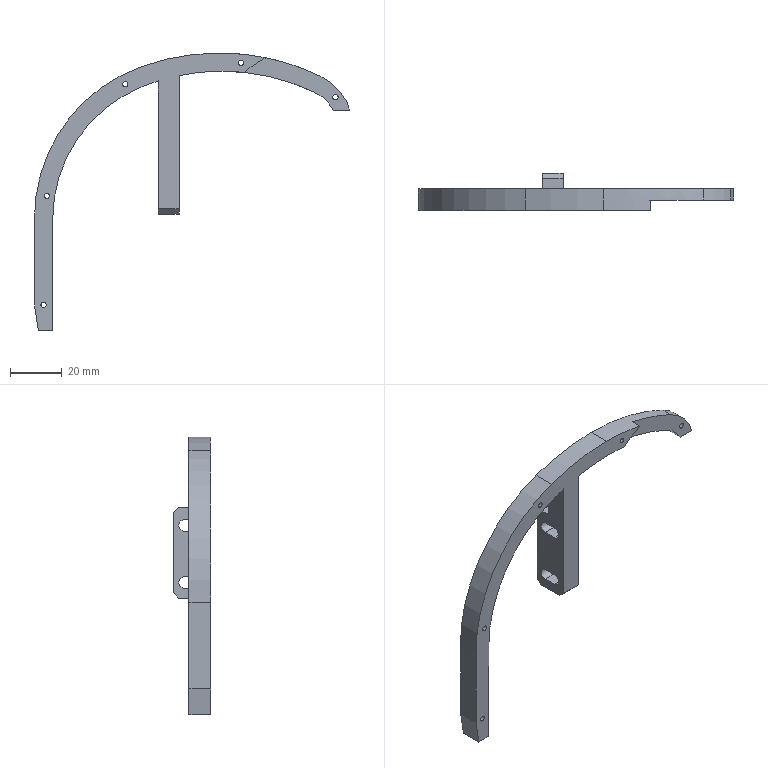Part | SolidWorks | features ICE 8, Chamfer 3, HoleWzd 2, Extrusion 1 | 1 solid | 45 faces | box 121.296 x 14.4 x 107 mm | volume 14940 mm3 | cylinder 24 | plane 21 | commonest cylinder face diameters 2.05 x10 4.5 x4 164.469 x3 178.469 x2 33 x1 47 x1
STEP:
#1=CARTESIAN_POINT('',(82.5,0.,-7.836));
#2=VERTEX_POINT('',#1);
#3=CARTESIAN_POINT('',(82.5,0.,-5.786));
#4=VERTEX_POINT('',#3);
#5=CARTESIAN_POINT('',(82.5,0.,-6.811));
#6=DIRECTION('',(0.,1.,0.));
#7=DIRECTION('',(0.,0.,1.));
#8=AXIS2_PLACEMENT_3D('',#5,#6,#7);
#9=CIRCLE('',#8,1.025);
#10=EDGE_CURVE('',#2,#4,#9,.T.);
#11=ORIENTED_EDGE('',*,*,#10,.F.);
#12=CARTESIAN_POINT('',(82.5,8.4,-7.836));
#13=VERTEX_POINT('',#12);
#14=CARTESIAN_POINT('',(82.5,8.4,-7.836));
#15=DIRECTION('',(0.,1.,0.));
#16=VECTOR('',#15,1000.);
#17=LINE('',#14,#16);
#18=EDGE_CURVE('',#2,#13,#17,.T.);
#19=ORIENTED_EDGE('',*,*,#18,.T.);
#20=CARTESIAN_POINT('',(82.5,8.4,-5.786));
#21=VERTEX_POINT('',#20);
#22=CARTESIAN_POINT('',(82.5,8.4,-6.811));
#23=DIRECTION('',(0.,1.,0.));
#24=DIRECTION('',(0.,0.,1.));
#25=AXIS2_PLACEMENT_3D('',#22,#23,#24);
#26=CIRCLE('',#25,1.025);
#27=EDGE_CURVE('',#13,#21,#26,.T.);
#28=ORIENTED_EDGE('',*,*,#27,.T.);
#29=CARTESIAN_POINT('',(82.5,8.4,-5.786));
#30=DIRECTION('',(0.,1.,0.));
#31=VECTOR('',#30,1000.);
#32=LINE('',#29,#31);
#33=EDGE_CURVE('',#4,#21,#32,.T.);
#34=ORIENTED_EDGE('',*,*,#33,.F.);
#35=EDGE_LOOP('',(#11,#19,#28,#34));
#36=FACE_OUTER_BOUND('',#35,.T.);
#37=CARTESIAN_POINT('',(82.5,8.4,-6.811));
#38=DIRECTION('',(0.,1.,0.));
#39=DIRECTION('',(0.,0.,1.));
#40=AXIS2_PLACEMENT_3D('',#37,#38,#39);
#41=CYLINDRICAL_SURFACE('',#40,1.025);
#42=ADVANCED_FACE('',(#36),#41,.F.);
#43=CARTESIAN_POINT('',(6.5,0.,-101.025));
#44=VERTEX_POINT('',#43);
#45=CARTESIAN_POINT('',(6.5,0.,-98.975));
#46=VERTEX_POINT('',#45);
#47=CARTESIAN_POINT('',(6.5,0.,-100.));
#48=DIRECTION('',(0.,1.,0.));
#49=DIRECTION('',(0.,0.,1.));
#50=AXIS2_PLACEMENT_3D('',#47,#48,#49);
#51=CIRCLE('',#50,1.025);
#52=EDGE_CURVE('',#44,#46,#51,.T.);
#53=ORIENTED_EDGE('',*,*,#52,.F.);
#54=CARTESIAN_POINT('',(6.5,8.4,-101.025));
#55=VERTEX_POINT('',#54);
#56=CARTESIAN_POINT('',(6.5,8.4,-101.025));
#57=DIRECTION('',(0.,1.,0.));
#58=VECTOR('',#57,1000.);
#59=LINE('',#56,#58);
#60=EDGE_CURVE('',#44,#55,#59,.T.);
#61=ORIENTED_EDGE('',*,*,#60,.T.);
#62=CARTESIAN_POINT('',(6.5,8.4,-98.975));
#63=VERTEX_POINT('',#62);
#64=CARTESIAN_POINT('',(6.5,8.4,-100.));
#65=DIRECTION('',(0.,1.,0.));
#66=DIRECTION('',(0.,0.,1.));
#67=AXIS2_PLACEMENT_3D('',#64,#65,#66);
#68=CIRCLE('',#67,1.025);
#69=EDGE_CURVE('',#55,#63,#68,.T.);
#70=ORIENTED_EDGE('',*,*,#69,.T.);
#71=CARTESIAN_POINT('',(6.5,8.4,-98.975));
#72=DIRECTION('',(0.,1.,0.));
#73=VECTOR('',#72,1000.);
#74=LINE('',#71,#73);
#75=EDGE_CURVE('',#46,#63,#74,.T.);
#76=ORIENTED_EDGE('',*,*,#75,.F.);
#77=EDGE_LOOP('',(#53,#61,#70,#76));
#78=FACE_OUTER_BOUND('',#77,.T.);
#79=CARTESIAN_POINT('',(6.5,8.4,-100.));
#80=DIRECTION('',(0.,1.,0.));
#81=DIRECTION('',(0.,0.,1.));
#82=AXIS2_PLACEMENT_3D('',#79,#80,#81);
#83=CYLINDRICAL_SURFACE('',#82,1.025);
#84=ADVANCED_FACE('',(#78),#83,.F.);
#85=CARTESIAN_POINT('',(7.74,0.,-59.025));
#86=VERTEX_POINT('',#85);
#87=CARTESIAN_POINT('',(7.74,0.,-56.975));
#88=VERTEX_POINT('',#87);
#89=CARTESIAN_POINT('',(7.74,0.,-58.));
#90=DIRECTION('',(0.,1.,0.));
#91=DIRECTION('',(0.,0.,1.));
#92=AXIS2_PLACEMENT_3D('',#89,#90,#91);
#93=CIRCLE('',#92,1.025);
#94=EDGE_CURVE('',#86,#88,#93,.T.);
#95=ORIENTED_EDGE('',*,*,#94,.F.);
#96=CARTESIAN_POINT('',(7.74,8.4,-59.025));
#97=VERTEX_POINT('',#96);
#98=CARTESIAN_POINT('',(7.74,8.4,-59.025));
#99=DIRECTION('',(0.,1.,0.));
#100=VECTOR('',#99,1000.);
#101=LINE('',#98,#100);
#102=EDGE_CURVE('',#86,#97,#101,.T.);
#103=ORIENTED_EDGE('',*,*,#102,.T.);
#104=CARTESIAN_POINT('',(7.74,8.4,-56.975));
#105=VERTEX_POINT('',#104);
#106=CARTESIAN_POINT('',(7.74,8.4,-58.));
#107=DIRECTION('',(0.,1.,0.));
#108=DIRECTION('',(0.,0.,1.));
#109=AXIS2_PLACEMENT_3D('',#106,#107,#108);
#110=CIRCLE('',#109,1.025);
#111=EDGE_CURVE('',#97,#105,#110,.T.);
#112=ORIENTED_EDGE('',*,*,#111,.T.);
#113=CARTESIAN_POINT('',(7.74,8.4,-56.975));
#114=DIRECTION('',(0.,1.,0.));
#115=VECTOR('',#114,1000.);
#116=LINE('',#113,#115);
#117=EDGE_CURVE('',#88,#105,#116,.T.);
#118=ORIENTED_EDGE('',*,*,#117,.F.);
#119=EDGE_LOOP('',(#95,#103,#112,#118));
#120=FACE_OUTER_BOUND('',#119,.T.);
#121=CARTESIAN_POINT('',(7.74,8.4,-58.));
#122=DIRECTION('',(0.,1.,0.));
#123=DIRECTION('',(0.,0.,1.));
#124=AXIS2_PLACEMENT_3D('',#121,#122,#123);
#125=CYLINDRICAL_SURFACE('',#124,1.025);
#126=ADVANCED_FACE('',(#120),#125,.F.);
#127=CARTESIAN_POINT('',(37.98,0.,-16.025));
#128=VERTEX_POINT('',#127);
#129=CARTESIAN_POINT('',(37.98,0.,-13.975));
#130=VERTEX_POINT('',#129);
#131=CARTESIAN_POINT('',(37.98,0.,-15.));
#132=DIRECTION('',(0.,1.,0.));
#133=DIRECTION('',(0.,0.,1.));
#134=AXIS2_PLACEMENT_3D('',#131,#132,#133);
#135=CIRCLE('',#134,1.025);
#136=EDGE_CURVE('',#128,#130,#135,.T.);
#137=ORIENTED_EDGE('',*,*,#136,.F.);
#138=CARTESIAN_POINT('',(37.98,8.4,-16.025));
#139=VERTEX_POINT('',#138);
#140=CARTESIAN_POINT('',(37.98,8.4,-16.025));
#141=DIRECTION('',(0.,1.,0.));
#142=VECTOR('',#141,1000.);
#143=LINE('',#140,#142);
#144=EDGE_CURVE('',#128,#139,#143,.T.);
#145=ORIENTED_EDGE('',*,*,#144,.T.);
#146=CARTESIAN_POINT('',(37.98,8.4,-13.975));
#147=VERTEX_POINT('',#146);
#148=CARTESIAN_POINT('',(37.98,8.4,-15.));
#149=DIRECTION('',(0.,1.,0.));
#150=DIRECTION('',(0.,0.,1.));
#151=AXIS2_PLACEMENT_3D('',#148,#149,#150);
#152=CIRCLE('',#151,1.025);
#153=EDGE_CURVE('',#139,#147,#152,.T.);
#154=ORIENTED_EDGE('',*,*,#153,.T.);
#155=CARTESIAN_POINT('',(37.98,8.4,-13.975));
#156=DIRECTION('',(0.,1.,0.));
#157=VECTOR('',#156,1000.);
#158=LINE('',#155,#157);
#159=EDGE_CURVE('',#130,#147,#158,.T.);
#160=ORIENTED_EDGE('',*,*,#159,.F.);
#161=EDGE_LOOP('',(#137,#145,#154,#160));
#162=FACE_OUTER_BOUND('',#161,.T.);
#163=CARTESIAN_POINT('',(37.98,8.4,-15.));
#164=DIRECTION('',(0.,1.,0.));
#165=DIRECTION('',(0.,0.,1.));
#166=AXIS2_PLACEMENT_3D('',#163,#164,#165);
#167=CYLINDRICAL_SURFACE('',#166,1.025);
#168=ADVANCED_FACE('',(#162),#167,.F.);
#169=CARTESIAN_POINT('',(118.899,4.,-18.975));
#170=VERTEX_POINT('',#169);
#171=CARTESIAN_POINT('',(118.899,4.,-21.025));
#172=VERTEX_POINT('',#171);
#173=CARTESIAN_POINT('',(118.899,4.,-20.));
#174=DIRECTION('',(0.,-1.,0.));
#175=DIRECTION('',(0.,0.,-1.));
#176=AXIS2_PLACEMENT_3D('',#173,#174,#175);
#177=CIRCLE('',#176,1.025);
#178=EDGE_CURVE('',#170,#172,#177,.T.);
#179=ORIENTED_EDGE('',*,*,#178,.T.);
#180=CARTESIAN_POINT('',(118.899,8.4,-21.025));
#181=VERTEX_POINT('',#180);
#182=CARTESIAN_POINT('',(118.899,8.4,-21.025));
#183=DIRECTION('',(0.,1.,0.));
#184=VECTOR('',#183,1000.);
#185=LINE('',#182,#184);
#186=EDGE_CURVE('',#172,#181,#185,.T.);
#187=ORIENTED_EDGE('',*,*,#186,.T.);
#188=CARTESIAN_POINT('',(118.899,8.4,-18.975));
#189=VERTEX_POINT('',#188);
#190=CARTESIAN_POINT('',(118.899,8.4,-20.));
#191=DIRECTION('',(0.,1.,0.));
#192=DIRECTION('',(0.,0.,1.));
#193=AXIS2_PLACEMENT_3D('',#190,#191,#192);
#194=CIRCLE('',#193,1.025);
#195=EDGE_CURVE('',#181,#189,#194,.T.);
#196=ORIENTED_EDGE('',*,*,#195,.T.);
#197=CARTESIAN_POINT('',(118.899,8.4,-18.975));
#198=DIRECTION('',(0.,1.,0.));
#199=VECTOR('',#198,1000.);
#200=LINE('',#197,#199);
#201=EDGE_CURVE('',#170,#189,#200,.T.);
#202=ORIENTED_EDGE('',*,*,#201,.F.);
#203=EDGE_LOOP('',(#179,#187,#196,#202));
#204=FACE_OUTER_BOUND('',#203,.T.);
#205=CARTESIAN_POINT('',(118.899,8.4,-20.));
#206=DIRECTION('',(0.,1.,0.));
#207=DIRECTION('',(0.,0.,1.));
#208=AXIS2_PLACEMENT_3D('',#205,#206,#207);
#209=CYLINDRICAL_SURFACE('',#208,1.025);
#210=ADVANCED_FACE('',(#204),#209,.F.);
#211=CARTESIAN_POINT('',(44.058,0.,-8.245));
#212=VERTEX_POINT('',#211);
#213=CARTESIAN_POINT('',(74.199,0.,-3.));
#214=VERTEX_POINT('',#213);
#215=CARTESIAN_POINT('',(74.199,0.,-92.234));
#216=DIRECTION('',(0.,1.,0.));
#217=DIRECTION('',(0.,0.,-1.));
#218=AXIS2_PLACEMENT_3D('',#215,#216,#217);
#219=CIRCLE('',#218,89.234);
#220=EDGE_CURVE('',#212,#214,#219,.T.);
#221=ORIENTED_EDGE('',*,*,#220,.T.);
#222=CARTESIAN_POINT('',(74.199,8.4,-3.));
#223=VERTEX_POINT('',#222);
#224=CARTESIAN_POINT('',(74.199,-22.6,-3.));
#225=DIRECTION('',(0.,1.,0.));
#226=VECTOR('',#225,1000.);
#227=LINE('',#224,#226);
#228=EDGE_CURVE('',#214,#223,#227,.T.);
#229=ORIENTED_EDGE('',*,*,#228,.T.);
#230=CARTESIAN_POINT('',(44.058,8.4,-8.245));
#231=VERTEX_POINT('',#230);
#232=CARTESIAN_POINT('',(74.199,8.4,-92.234));
#233=DIRECTION('',(0.,-1.,0.));
#234=DIRECTION('',(0.,0.,1.));
#235=AXIS2_PLACEMENT_3D('',#232,#233,#234);
#236=CIRCLE('',#235,89.234);
#237=EDGE_CURVE('',#223,#231,#236,.T.);
#238=ORIENTED_EDGE('',*,*,#237,.T.);
#239=CARTESIAN_POINT('',(44.058,-22.6,-8.245));
#240=DIRECTION('',(0.,1.,0.));
#241=VECTOR('',#240,1000.);
#242=LINE('',#239,#241);
#243=EDGE_CURVE('',#212,#231,#242,.T.);
#244=ORIENTED_EDGE('',*,*,#243,.F.);
#245=EDGE_LOOP('',(#221,#229,#238,#244));
#246=FACE_OUTER_BOUND('',#245,.T.);
#247=CARTESIAN_POINT('',(74.199,-22.6,-92.234));
#248=DIRECTION('',(0.,1.,0.));
#249=DIRECTION('',(0.,0.,1.));
#250=AXIS2_PLACEMENT_3D('',#247,#248,#249);
#251=CYLINDRICAL_SURFACE('',#250,89.234);
#252=ADVANCED_FACE('',(#246),#251,.T.);
#253=CARTESIAN_POINT('',(75.199,0.,-10.));
#254=VERTEX_POINT('',#253);
#255=CARTESIAN_POINT('',(83.777,0.,-10.449));
#256=VERTEX_POINT('',#255);
#257=CARTESIAN_POINT('',(75.199,0.,-92.234));
#258=DIRECTION('',(0.,1.,0.));
#259=DIRECTION('',(0.,0.,1.));
#260=AXIS2_PLACEMENT_3D('',#257,#258,#259);
#261=CIRCLE('',#260,82.234);
#262=EDGE_CURVE('',#254,#256,#261,.T.);
#263=ORIENTED_EDGE('',*,*,#262,.F.);
#264=CARTESIAN_POINT('',(75.199,8.4,-10.));
#265=VERTEX_POINT('',#264);
#266=CARTESIAN_POINT('',(75.199,0.,-10.));
#267=DIRECTION('',(0.,1.,0.));
#268=VECTOR('',#267,1000.);
#269=LINE('',#266,#268);
#270=EDGE_CURVE('',#254,#265,#269,.T.);
#271=ORIENTED_EDGE('',*,*,#270,.T.);
#272=CARTESIAN_POINT('',(110.854,8.4,-18.132));
#273=VERTEX_POINT('',#272);
#274=CARTESIAN_POINT('',(75.199,8.4,-92.234));
#275=DIRECTION('',(0.,-1.,0.));
#276=DIRECTION('',(0.,0.,1.));
#277=AXIS2_PLACEMENT_3D('',#274,#275,#276);
#278=CIRCLE('',#277,82.234);
#279=EDGE_CURVE('',#273,#265,#278,.T.);
#280=ORIENTED_EDGE('',*,*,#279,.F.);
#281=CARTESIAN_POINT('',(110.854,4.,-18.132));
#282=VERTEX_POINT('',#281);
#283=CARTESIAN_POINT('',(110.854,0.,-18.132));
#284=DIRECTION('',(0.,1.,0.));
#285=VECTOR('',#284,1000.);
#286=LINE('',#283,#285);
#287=EDGE_CURVE('',#282,#273,#286,.T.);
#288=ORIENTED_EDGE('',*,*,#287,.F.);
#289=CARTESIAN_POINT('',(83.777,4.,-10.449));
#290=VERTEX_POINT('',#289);
#291=CARTESIAN_POINT('',(75.199,4.,-92.234));
#292=DIRECTION('',(0.,1.,0.));
#293=DIRECTION('',(0.,0.,-1.));
#294=AXIS2_PLACEMENT_3D('',#291,#292,#293);
#295=CIRCLE('',#294,82.234);
#296=EDGE_CURVE('',#290,#282,#295,.T.);
#297=ORIENTED_EDGE('',*,*,#296,.F.);
#298=CARTESIAN_POINT('',(83.777,2.,-10.449));
#299=DIRECTION('',(0.,-1.,0.));
#300=VECTOR('',#299,1000.);
#301=LINE('',#298,#300);
#302=EDGE_CURVE('',#290,#256,#301,.T.);
#303=ORIENTED_EDGE('',*,*,#302,.T.);
#304=EDGE_LOOP('',(#263,#271,#280,#288,#297,#303));
#305=FACE_OUTER_BOUND('',#304,.T.);
#306=CARTESIAN_POINT('',(75.199,0.,-92.234));
#307=DIRECTION('',(0.,1.,0.));
#308=DIRECTION('',(0.,0.,1.));
#309=AXIS2_PLACEMENT_3D('',#306,#307,#308);
#310=CYLINDRICAL_SURFACE('',#309,82.234);
#311=ADVANCED_FACE('',(#305),#310,.F.);
#312=CARTESIAN_POINT('',(118.131,4.,-25.));
#313=VERTEX_POINT('',#312);
#314=CARTESIAN_POINT('',(103.7,4.,-33.));
#315=DIRECTION('',(0.,1.,0.));
#316=DIRECTION('',(0.,0.,-1.));
#317=AXIS2_PLACEMENT_3D('',#314,#315,#316);
#318=CIRCLE('',#317,16.5);
#319=EDGE_CURVE('',#282,#313,#318,.T.);
#320=ORIENTED_EDGE('',*,*,#319,.F.);
#321=ORIENTED_EDGE('',*,*,#287,.T.);
#322=CARTESIAN_POINT('',(118.131,8.4,-25.));
#323=VERTEX_POINT('',#322);
#324=CARTESIAN_POINT('',(103.7,8.4,-33.));
#325=DIRECTION('',(0.,-1.,0.));
#326=DIRECTION('',(0.,0.,1.));
#327=AXIS2_PLACEMENT_3D('',#324,#325,#326);
#328=CIRCLE('',#327,16.5);
#329=EDGE_CURVE('',#323,#273,#328,.T.);
#330=ORIENTED_EDGE('',*,*,#329,.F.);
#331=CARTESIAN_POINT('',(118.131,0.,-25.));
#332=DIRECTION('',(0.,-1.,0.));
#333=VECTOR('',#332,1000.);
#334=LINE('',#331,#333);
#335=EDGE_CURVE('',#323,#313,#334,.T.);
#336=ORIENTED_EDGE('',*,*,#335,.T.);
#337=EDGE_LOOP('',(#320,#321,#330,#336));
#338=FACE_OUTER_BOUND('',#337,.T.);
#339=CARTESIAN_POINT('',(103.7,0.,-33.));
#340=DIRECTION('',(0.,1.,0.));
#341=DIRECTION('',(0.,0.,1.));
#342=AXIS2_PLACEMENT_3D('',#339,#340,#341);
#343=CYLINDRICAL_SURFACE('',#342,16.5);
#344=ADVANCED_FACE('',(#338),#343,.F.);
#345=CARTESIAN_POINT('',(124.296,8.4,-25.));
#346=VERTEX_POINT('',#345);
#347=CARTESIAN_POINT('',(130.,8.4,-25.));
#348=DIRECTION('',(-1.,0.,0.));
#349=VECTOR('',#348,1000.);
#350=LINE('',#347,#349);
#351=EDGE_CURVE('',#346,#323,#350,.T.);
#352=ORIENTED_EDGE('',*,*,#351,.F.);
#353=CARTESIAN_POINT('',(124.296,4.,-25.));
#354=VERTEX_POINT('',#353);
#355=CARTESIAN_POINT('',(124.296,0.,-25.));
#356=DIRECTION('',(0.,-1.,0.));
#357=VECTOR('',#356,1000.);
#358=LINE('',#355,#357);
#359=EDGE_CURVE('',#346,#354,#358,.T.);
#360=ORIENTED_EDGE('',*,*,#359,.T.);
#361=CARTESIAN_POINT('',(130.,4.,-25.));
#362=DIRECTION('',(1.,0.,0.));
#363=VECTOR('',#362,1000.);
#364=LINE('',#361,#363);
#365=EDGE_CURVE('',#313,#354,#364,.T.);
#366=ORIENTED_EDGE('',*,*,#365,.F.);
#367=ORIENTED_EDGE('',*,*,#335,.F.);
#368=EDGE_LOOP('',(#352,#360,#366,#367));
#369=FACE_OUTER_BOUND('',#368,.T.);
#370=CARTESIAN_POINT('',(130.,0.,-25.));
#371=DIRECTION('',(0.,0.,1.));
#372=DIRECTION('',(1.,0.,0.));
#373=AXIS2_PLACEMENT_3D('',#370,#371,#372);
#374=PLANE('',#373);
#375=ADVANCED_FACE('',(#369),#374,.F.);
#376=CARTESIAN_POINT('',(123.242,4.,-21.586));
#377=VERTEX_POINT('',#376);
#378=CARTESIAN_POINT('',(112.889,4.,-11.824));
#379=VERTEX_POINT('',#378);
#380=CARTESIAN_POINT('',(102.7,4.,-33.));
#381=DIRECTION('',(0.,-1.,0.));
#382=DIRECTION('',(0.,0.,-1.));
#383=AXIS2_PLACEMENT_3D('',#380,#381,#382);
#384=CIRCLE('',#383,23.5);
#385=EDGE_CURVE('',#377,#379,#384,.T.);
#386=ORIENTED_EDGE('',*,*,#385,.F.);
#387=CARTESIAN_POINT('',(123.242,8.4,-21.586));
#388=VERTEX_POINT('',#387);
#389=CARTESIAN_POINT('',(123.242,-22.6,-21.586));
#390=DIRECTION('',(0.,1.,0.));
#391=VECTOR('',#390,1000.);
#392=LINE('',#389,#391);
#393=EDGE_CURVE('',#377,#388,#392,.T.);
#394=ORIENTED_EDGE('',*,*,#393,.T.);
#395=CARTESIAN_POINT('',(112.889,8.4,-11.824));
#396=VERTEX_POINT('',#395);
#397=CARTESIAN_POINT('',(102.7,8.4,-33.));
#398=DIRECTION('',(0.,-1.,0.));
#399=DIRECTION('',(0.,0.,1.));
#400=AXIS2_PLACEMENT_3D('',#397,#398,#399);
#401=CIRCLE('',#400,23.5);
#402=EDGE_CURVE('',#388,#396,#401,.T.);
#403=ORIENTED_EDGE('',*,*,#402,.T.);
#404=CARTESIAN_POINT('',(112.889,-22.6,-11.824));
#405=DIRECTION('',(0.,1.,0.));
#406=VECTOR('',#405,1000.);
#407=LINE('',#404,#406);
#408=EDGE_CURVE('',#379,#396,#407,.T.);
#409=ORIENTED_EDGE('',*,*,#408,.F.);
#410=EDGE_LOOP('',(#386,#394,#403,#409));
#411=FACE_OUTER_BOUND('',#410,.T.);
#412=CARTESIAN_POINT('',(102.7,-22.6,-33.));
#413=DIRECTION('',(0.,1.,0.));
#414=DIRECTION('',(0.,0.,1.));
#415=AXIS2_PLACEMENT_3D('',#412,#413,#414);
#416=CYLINDRICAL_SURFACE('',#415,23.5);
#417=ADVANCED_FACE('',(#411),#416,.T.);
#418=CARTESIAN_POINT('',(50.7,8.4,-13.734));
#419=VERTEX_POINT('',#418);
#420=CARTESIAN_POINT('',(44.403,8.4,-15.984));
#421=VERTEX_POINT('',#420);
#422=CARTESIAN_POINT('',(75.199,8.4,-92.234));
#423=DIRECTION('',(0.,-1.,0.));
#424=DIRECTION('',(0.,0.,1.));
#425=AXIS2_PLACEMENT_3D('',#422,#423,#424);
#426=CIRCLE('',#425,82.234);
#427=EDGE_CURVE('',#419,#421,#426,.T.);
#428=ORIENTED_EDGE('',*,*,#427,.F.);
#429=CARTESIAN_POINT('',(50.7,0.,-13.734));
#430=VERTEX_POINT('',#429);
#431=CARTESIAN_POINT('',(50.7,-53.925,-13.734));
#432=DIRECTION('',(0.,1.,0.));
#433=VECTOR('',#432,1000.);
#434=LINE('',#431,#433);
#435=EDGE_CURVE('',#430,#419,#434,.T.);
#436=ORIENTED_EDGE('',*,*,#435,.F.);
#437=CARTESIAN_POINT('',(44.403,0.,-15.984));
#438=VERTEX_POINT('',#437);
#439=CARTESIAN_POINT('',(75.199,0.,-92.234));
#440=DIRECTION('',(0.,1.,0.));
#441=DIRECTION('',(0.,0.,1.));
#442=AXIS2_PLACEMENT_3D('',#439,#440,#441);
#443=CIRCLE('',#442,82.234);
#444=EDGE_CURVE('',#438,#430,#443,.T.);
#445=ORIENTED_EDGE('',*,*,#444,.F.);
#446=CARTESIAN_POINT('',(44.403,0.,-15.984));
#447=DIRECTION('',(0.,1.,0.));
#448=VECTOR('',#447,1000.);
#449=LINE('',#446,#448);
#450=EDGE_CURVE('',#438,#421,#449,.T.);
#451=ORIENTED_EDGE('',*,*,#450,.T.);
#452=EDGE_LOOP('',(#428,#436,#445,#451));
#453=FACE_OUTER_BOUND('',#452,.T.);
#454=CARTESIAN_POINT('',(75.199,0.,-92.234));
#455=DIRECTION('',(0.,1.,0.));
#456=DIRECTION('',(0.,0.,1.));
#457=AXIS2_PLACEMENT_3D('',#454,#455,#456);
#458=CYLINDRICAL_SURFACE('',#457,82.234);
#459=ADVANCED_FACE('',(#453),#458,.F.);
#460=CARTESIAN_POINT('',(10.,0.,-110.));
#461=VERTEX_POINT('',#460);
#462=CARTESIAN_POINT('',(4.5,0.,-110.));
#463=VERTEX_POINT('',#462);
#464=CARTESIAN_POINT('',(0.,0.,-110.));
#465=DIRECTION('',(-1.,0.,0.));
#466=VECTOR('',#465,1000.);
#467=LINE('',#464,#466);
#468=EDGE_CURVE('',#461,#463,#467,.T.);
#469=ORIENTED_EDGE('',*,*,#468,.T.);
#470=CARTESIAN_POINT('',(4.5,8.4,-110.));
#471=VERTEX_POINT('',#470);
#472=CARTESIAN_POINT('',(4.5,14.4,-110.));
#473=DIRECTION('',(0.,1.,0.));
#474=VECTOR('',#473,1000.);
#475=LINE('',#472,#474);
#476=EDGE_CURVE('',#463,#471,#475,.T.);
#477=ORIENTED_EDGE('',*,*,#476,.T.);
#478=CARTESIAN_POINT('',(10.,8.4,-110.));
#479=VERTEX_POINT('',#478);
#480=CARTESIAN_POINT('',(0.,8.4,-110.));
#481=DIRECTION('',(-1.,0.,0.));
#482=VECTOR('',#481,1000.);
#483=LINE('',#480,#482);
#484=EDGE_CURVE('',#479,#471,#483,.T.);
#485=ORIENTED_EDGE('',*,*,#484,.F.);
#486=CARTESIAN_POINT('',(10.,0.,-110.));
#487=DIRECTION('',(0.,1.,0.));
#488=VECTOR('',#487,1000.);
#489=LINE('',#486,#488);
#490=EDGE_CURVE('',#461,#479,#489,.T.);
#491=ORIENTED_EDGE('',*,*,#490,.F.);
#492=EDGE_LOOP('',(#469,#477,#485,#491));
#493=FACE_OUTER_BOUND('',#492,.T.);
#494=CARTESIAN_POINT('',(0.,14.4,-110.));
#495=DIRECTION('',(0.,0.,1.));
#496=DIRECTION('',(1.,0.,0.));
#497=AXIS2_PLACEMENT_3D('',#494,#495,#496);
#498=PLANE('',#497);
#499=ADVANCED_FACE('',(#493),#498,.F.);
#500=CARTESIAN_POINT('',(50.7,14.4,-63.));
#501=VERTEX_POINT('',#500);
#502=CARTESIAN_POINT('',(50.7,14.4,-32.));
#503=VERTEX_POINT('',#502);
#504=CARTESIAN_POINT('',(50.7,14.4,-13.734));
#505=DIRECTION('',(0.,0.,1.));
#506=VECTOR('',#505,1000.);
#507=LINE('',#504,#506);
#508=EDGE_CURVE('',#501,#503,#507,.T.);
#509=ORIENTED_EDGE('',*,*,#508,.T.);
#510=CARTESIAN_POINT('',(58.7,14.4,-32.));
#511=VERTEX_POINT('',#510);
#512=CARTESIAN_POINT('',(58.7,14.4,-32.));
#513=DIRECTION('',(1.,0.,0.));
#514=VECTOR('',#513,1000.);
#515=LINE('',#512,#514);
#516=EDGE_CURVE('',#503,#511,#515,.T.);
#517=ORIENTED_EDGE('',*,*,#516,.T.);
#518=CARTESIAN_POINT('',(58.7,14.4,-63.));
#519=VERTEX_POINT('',#518);
#520=CARTESIAN_POINT('',(58.7,14.4,-11.672));
#521=DIRECTION('',(0.,0.,-1.));
#522=VECTOR('',#521,1000.);
#523=LINE('',#520,#522);
#524=EDGE_CURVE('',#511,#519,#523,.T.);
#525=ORIENTED_EDGE('',*,*,#524,.T.);
#526=CARTESIAN_POINT('',(50.7,14.4,-63.));
#527=DIRECTION('',(-1.,0.,0.));
#528=VECTOR('',#527,1000.);
#529=LINE('',#526,#528);
#530=EDGE_CURVE('',#519,#501,#529,.T.);
#531=ORIENTED_EDGE('',*,*,#530,.T.);
#532=EDGE_LOOP('',(#509,#517,#525,#531));
#533=FACE_OUTER_BOUND('',#532,.T.);
#534=CARTESIAN_POINT('',(0.,14.4,0.));
#535=DIRECTION('',(0.,-1.,0.));
#536=DIRECTION('',(0.,0.,-1.));
#537=AXIS2_PLACEMENT_3D('',#534,#535,#536);
#538=PLANE('',#537);
#539=ADVANCED_FACE('',(#533),#538,.F.);
#540=ORIENTED_EDGE('',*,*,#270,.F.);
#541=CARTESIAN_POINT('',(58.7,0.,-11.672));
#542=VERTEX_POINT('',#541);
#543=CARTESIAN_POINT('',(75.199,0.,-92.234));
#544=DIRECTION('',(0.,1.,0.));
#545=DIRECTION('',(0.,0.,1.));
#546=AXIS2_PLACEMENT_3D('',#543,#544,#545);
#547=CIRCLE('',#546,82.234);
#548=EDGE_CURVE('',#542,#254,#547,.T.);
#549=ORIENTED_EDGE('',*,*,#548,.F.);
#550=CARTESIAN_POINT('',(58.7,8.4,-11.672));
#551=VERTEX_POINT('',#550);
#552=CARTESIAN_POINT('',(58.7,-53.925,-11.672));
#553=DIRECTION('',(0.,1.,0.));
#554=VECTOR('',#553,1000.);
#555=LINE('',#552,#554);
#556=EDGE_CURVE('',#542,#551,#555,.T.);
#557=ORIENTED_EDGE('',*,*,#556,.T.);
#558=CARTESIAN_POINT('',(75.199,8.4,-92.234));
#559=DIRECTION('',(0.,-1.,0.));
#560=DIRECTION('',(0.,0.,1.));
#561=AXIS2_PLACEMENT_3D('',#558,#559,#560);
#562=CIRCLE('',#561,82.234);
#563=EDGE_CURVE('',#265,#551,#562,.T.);
#564=ORIENTED_EDGE('',*,*,#563,.F.);
#565=EDGE_LOOP('',(#540,#549,#557,#564));
#566=FACE_OUTER_BOUND('',#565,.T.);
#567=CARTESIAN_POINT('',(75.199,0.,-92.234));
#568=DIRECTION('',(0.,1.,0.));
#569=DIRECTION('',(0.,0.,1.));
#570=AXIS2_PLACEMENT_3D('',#567,#568,#569);
#571=CYLINDRICAL_SURFACE('',#570,82.234);
#572=ADVANCED_FACE('',(#566),#571,.F.);
#573=CARTESIAN_POINT('',(10.,8.4,-66.982));
#574=VERTEX_POINT('',#573);
#575=CARTESIAN_POINT('',(65.,8.4,-66.982));
#576=DIRECTION('',(0.,-1.,0.));
#577=DIRECTION('',(0.,0.,1.));
#578=AXIS2_PLACEMENT_3D('',#575,#576,#577);
#579=CIRCLE('',#578,55.);
#580=EDGE_CURVE('',#421,#574,#579,.T.);
#581=ORIENTED_EDGE('',*,*,#580,.F.);
#582=ORIENTED_EDGE('',*,*,#450,.F.);
#583=CARTESIAN_POINT('',(10.,0.,-66.982));
#584=VERTEX_POINT('',#583);
#585=CARTESIAN_POINT('',(65.,0.,-66.982));
#586=DIRECTION('',(0.,1.,0.));
#587=DIRECTION('',(0.,0.,1.));
#588=AXIS2_PLACEMENT_3D('',#585,#586,#587);
#589=CIRCLE('',#588,55.);
#590=EDGE_CURVE('',#584,#438,#589,.T.);
#591=ORIENTED_EDGE('',*,*,#590,.F.);
#592=CARTESIAN_POINT('',(10.,0.,-66.982));
#593=DIRECTION('',(0.,1.,0.));
#594=VECTOR('',#593,1000.);
#595=LINE('',#592,#594);
#596=EDGE_CURVE('',#584,#574,#595,.T.);
#597=ORIENTED_EDGE('',*,*,#596,.T.);
#598=EDGE_LOOP('',(#581,#582,#591,#597));
#599=FACE_OUTER_BOUND('',#598,.T.);
#600=CARTESIAN_POINT('',(65.,0.,-66.982));
#601=DIRECTION('',(0.,1.,0.));
#602=DIRECTION('',(0.,0.,1.));
#603=AXIS2_PLACEMENT_3D('',#600,#601,#602);
#604=CYLINDRICAL_SURFACE('',#603,55.);
#605=ADVANCED_FACE('',(#599),#604,.F.);
#606=CARTESIAN_POINT('',(10.,8.4,-110.));
#607=DIRECTION('',(0.,0.,-1.));
#608=VECTOR('',#607,1000.);
#609=LINE('',#606,#608);
#610=EDGE_CURVE('',#574,#479,#609,.T.);
#611=ORIENTED_EDGE('',*,*,#610,.F.);
#612=ORIENTED_EDGE('',*,*,#596,.F.);
#613=CARTESIAN_POINT('',(10.,0.,-110.));
#614=DIRECTION('',(0.,0.,1.));
#615=VECTOR('',#614,1000.);
#616=LINE('',#613,#615);
#617=EDGE_CURVE('',#461,#584,#616,.T.);
#618=ORIENTED_EDGE('',*,*,#617,.F.);
#619=ORIENTED_EDGE('',*,*,#490,.T.);
#620=EDGE_LOOP('',(#611,#612,#618,#619));
#621=FACE_OUTER_BOUND('',#620,.T.);
#622=CARTESIAN_POINT('',(10.,0.,-110.));
#623=DIRECTION('',(-1.,0.,0.));
#624=DIRECTION('',(0.,0.,1.));
#625=AXIS2_PLACEMENT_3D('',#622,#623,#624);
#626=PLANE('',#625);
#627=ADVANCED_FACE('',(#621),#626,.F.);
#628=CARTESIAN_POINT('',(58.7,10.,-39.25));
#629=VERTEX_POINT('',#628);
#630=CARTESIAN_POINT('',(58.7,10.,-34.75));
#631=VERTEX_POINT('',#630);
#632=CARTESIAN_POINT('',(58.7,10.,-37.));
#633=DIRECTION('',(1.,0.,0.));
#634=DIRECTION('',(0.,0.,-1.));
#635=AXIS2_PLACEMENT_3D('',#632,#633,#634);
#636=CIRCLE('',#635,2.25);
#637=EDGE_CURVE('',#629,#631,#636,.T.);
#638=ORIENTED_EDGE('',*,*,#637,.F.);
#639=CARTESIAN_POINT('',(58.7,5.,-39.25));
#640=VERTEX_POINT('',#639);
#641=CARTESIAN_POINT('',(58.7,10.,-39.25));
#642=DIRECTION('',(0.,1.,0.));
#643=VECTOR('',#642,1000.);
#644=LINE('',#641,#643);
#645=EDGE_CURVE('',#640,#629,#644,.T.);
#646=ORIENTED_EDGE('',*,*,#645,.F.);
#647=CARTESIAN_POINT('',(58.7,5.,-34.75));
#648=VERTEX_POINT('',#647);
#649=CARTESIAN_POINT('',(58.7,5.,-37.));
#650=DIRECTION('',(1.,0.,0.));
#651=DIRECTION('',(0.,0.,-1.));
#652=AXIS2_PLACEMENT_3D('',#649,#650,#651);
#653=CIRCLE('',#652,2.25);
#654=EDGE_CURVE('',#648,#640,#653,.T.);
#655=ORIENTED_EDGE('',*,*,#654,.F.);
#656=CARTESIAN_POINT('',(58.7,10.,-34.75));
#657=DIRECTION('',(0.,-1.,0.));
#658=VECTOR('',#657,1000.);
#659=LINE('',#656,#658);
#660=EDGE_CURVE('',#631,#648,#659,.T.);
#661=ORIENTED_EDGE('',*,*,#660,.F.);
#662=EDGE_LOOP('',(#638,#646,#655,#661));
#663=FACE_BOUND('',#662,.T.);
#664=CARTESIAN_POINT('',(58.7,10.,-61.25));
#665=VERTEX_POINT('',#664);
#666=CARTESIAN_POINT('',(58.7,10.,-56.75));
#667=VERTEX_POINT('',#666);
#668=CARTESIAN_POINT('',(58.7,10.,-59.));
#669=DIRECTION('',(1.,0.,0.));
#670=DIRECTION('',(0.,0.,-1.));
#671=AXIS2_PLACEMENT_3D('',#668,#669,#670);
#672=CIRCLE('',#671,2.25);
#673=EDGE_CURVE('',#665,#667,#672,.T.);
#674=ORIENTED_EDGE('',*,*,#673,.F.);
#675=CARTESIAN_POINT('',(58.7,5.,-61.25));
#676=VERTEX_POINT('',#675);
#677=CARTESIAN_POINT('',(58.7,10.,-61.25));
#678=DIRECTION('',(0.,1.,0.));
#679=VECTOR('',#678,1000.);
#680=LINE('',#677,#679);
#681=EDGE_CURVE('',#676,#665,#680,.T.);
#682=ORIENTED_EDGE('',*,*,#681,.F.);
#683=CARTESIAN_POINT('',(58.7,5.,-56.75));
#684=VERTEX_POINT('',#683);
#685=CARTESIAN_POINT('',(58.7,5.,-59.));
#686=DIRECTION('',(1.,0.,0.));
#687=DIRECTION('',(0.,0.,-1.));
#688=AXIS2_PLACEMENT_3D('',#685,#686,#687);
#689=CIRCLE('',#688,2.25);
#690=EDGE_CURVE('',#684,#676,#689,.T.);
#691=ORIENTED_EDGE('',*,*,#690,.F.);
#692=CARTESIAN_POINT('',(58.7,10.,-56.75));
#693=DIRECTION('',(0.,-1.,0.));
#694=VECTOR('',#693,1000.);
#695=LINE('',#692,#694);
#696=EDGE_CURVE('',#667,#684,#695,.T.);
#697=ORIENTED_EDGE('',*,*,#696,.F.);
#698=EDGE_LOOP('',(#674,#682,#691,#697));
#699=FACE_BOUND('',#698,.T.);
#700=CARTESIAN_POINT('',(58.7,0.,-63.));
#701=VERTEX_POINT('',#700);
#702=CARTESIAN_POINT('',(58.7,0.,-11.672));
#703=DIRECTION('',(0.,0.,-1.));
#704=VECTOR('',#703,1000.);
#705=LINE('',#702,#704);
#706=EDGE_CURVE('',#542,#701,#705,.T.);
#707=ORIENTED_EDGE('',*,*,#706,.T.);
#708=CARTESIAN_POINT('',(58.7,2.,-65.));
#709=VERTEX_POINT('',#708);
#710=CARTESIAN_POINT('',(58.7,-52.626,-10.374));
#711=DIRECTION('',(0.,0.7071,-0.7071));
#712=VECTOR('',#711,1000.);
#713=LINE('',#710,#712);
#714=EDGE_CURVE('',#701,#709,#713,.T.);
#715=ORIENTED_EDGE('',*,*,#714,.T.);
#716=CARTESIAN_POINT('',(58.7,12.4,-65.));
#717=VERTEX_POINT('',#716);
#718=CARTESIAN_POINT('',(58.7,-53.925,-65.));
#719=DIRECTION('',(0.,1.,0.));
#720=VECTOR('',#719,1000.);
#721=LINE('',#718,#720);
#722=EDGE_CURVE('',#709,#717,#721,.T.);
#723=ORIENTED_EDGE('',*,*,#722,.T.);
#724=CARTESIAN_POINT('',(58.7,5.902,-71.498));
#725=DIRECTION('',(0.,0.7071,0.7071));
#726=VECTOR('',#725,1000.);
#727=LINE('',#724,#726);
#728=EDGE_CURVE('',#717,#519,#727,.T.);
#729=ORIENTED_EDGE('',*,*,#728,.T.);
#730=ORIENTED_EDGE('',*,*,#524,.F.);
#731=CARTESIAN_POINT('',(58.7,12.4,-30.));
#732=VERTEX_POINT('',#731);
#733=CARTESIAN_POINT('',(58.7,-29.926,12.326));
#734=DIRECTION('',(0.,-0.7071,0.7071));
#735=VECTOR('',#734,1000.);
#736=LINE('',#733,#735);
#737=EDGE_CURVE('',#511,#732,#736,.T.);
#738=ORIENTED_EDGE('',*,*,#737,.T.);
#739=CARTESIAN_POINT('',(58.7,8.4,-30.));
#740=VERTEX_POINT('',#739);
#741=CARTESIAN_POINT('',(58.7,8.4,-30.));
#742=DIRECTION('',(0.,1.,0.));
#743=VECTOR('',#742,1000.);
#744=LINE('',#741,#743);
#745=EDGE_CURVE('',#740,#732,#744,.T.);
#746=ORIENTED_EDGE('',*,*,#745,.F.);
#747=CARTESIAN_POINT('',(58.7,8.4,-11.672));
#748=DIRECTION('',(0.,0.,1.));
#749=VECTOR('',#748,1000.);
#750=LINE('',#747,#749);
#751=EDGE_CURVE('',#740,#551,#750,.T.);
#752=ORIENTED_EDGE('',*,*,#751,.T.);
#753=ORIENTED_EDGE('',*,*,#556,.F.);
#754=EDGE_LOOP('',(#707,#715,#723,#729,#730,#738,#746,#752,#753));
#755=FACE_OUTER_BOUND('',#754,.T.);
#756=CARTESIAN_POINT('',(58.7,-53.925,-11.672));
#757=DIRECTION('',(1.,0.,0.));
#758=DIRECTION('',(0.,0.,-1.));
#759=AXIS2_PLACEMENT_3D('',#756,#757,#758);
#760=PLANE('',#759);
#761=ADVANCED_FACE('',(#663,#699,#755),#760,.T.);
#762=CARTESIAN_POINT('',(82.5,0.,-6.811));
#763=DIRECTION('',(0.,1.,0.));
#764=DIRECTION('',(0.,0.,1.));
#765=AXIS2_PLACEMENT_3D('',#762,#763,#764);
#766=CIRCLE('',#765,1.025);
#767=EDGE_CURVE('',#4,#2,#766,.T.);
#768=ORIENTED_EDGE('',*,*,#767,.T.);
#769=ORIENTED_EDGE('',*,*,#10,.T.);
#770=EDGE_LOOP('',(#768,#769));
#771=FACE_BOUND('',#770,.T.);
#772=CARTESIAN_POINT('',(6.5,0.,-100.));
#773=DIRECTION('',(0.,1.,0.));
#774=DIRECTION('',(0.,0.,1.));
#775=AXIS2_PLACEMENT_3D('',#772,#773,#774);
#776=CIRCLE('',#775,1.025);
#777=EDGE_CURVE('',#46,#44,#776,.T.);
#778=ORIENTED_EDGE('',*,*,#777,.T.);
#779=ORIENTED_EDGE('',*,*,#52,.T.);
#780=EDGE_LOOP('',(#778,#779));
#781=FACE_BOUND('',#780,.T.);
#782=CARTESIAN_POINT('',(7.74,0.,-58.));
#783=DIRECTION('',(0.,1.,0.));
#784=DIRECTION('',(0.,0.,1.));
#785=AXIS2_PLACEMENT_3D('',#782,#783,#784);
#786=CIRCLE('',#785,1.025);
#787=EDGE_CURVE('',#88,#86,#786,.T.);
#788=ORIENTED_EDGE('',*,*,#787,.T.);
#789=ORIENTED_EDGE('',*,*,#94,.T.);
#790=EDGE_LOOP('',(#788,#789));
#791=FACE_BOUND('',#790,.T.);
#792=CARTESIAN_POINT('',(37.98,0.,-15.));
#793=DIRECTION('',(0.,1.,0.));
#794=DIRECTION('',(0.,0.,1.));
#795=AXIS2_PLACEMENT_3D('',#792,#793,#794);
#796=CIRCLE('',#795,1.025);
#797=EDGE_CURVE('',#130,#128,#796,.T.);
#798=ORIENTED_EDGE('',*,*,#797,.T.);
#799=ORIENTED_EDGE('',*,*,#136,.T.);
#800=EDGE_LOOP('',(#798,#799));
#801=FACE_BOUND('',#800,.T.);
#802=CARTESIAN_POINT('',(3.,0.,-100.));
#803=VERTEX_POINT('',#802);
#804=CARTESIAN_POINT('',(3.,0.,-66.601));
#805=VERTEX_POINT('',#804);
#806=CARTESIAN_POINT('',(3.,0.,0.));
#807=DIRECTION('',(0.,0.,1.));
#808=VECTOR('',#807,1000.);
#809=LINE('',#806,#808);
#810=EDGE_CURVE('',#803,#805,#809,.T.);
#811=ORIENTED_EDGE('',*,*,#810,.F.);
#812=CARTESIAN_POINT('',(-11.736,0.,-1.76));
#813=DIRECTION('',(0.1483,0.,-0.9889));
#814=VECTOR('',#813,1000.);
#815=LINE('',#812,#814);
#816=EDGE_CURVE('',#803,#463,#815,.T.);
#817=ORIENTED_EDGE('',*,*,#816,.T.);
#818=ORIENTED_EDGE('',*,*,#468,.F.);
#819=ORIENTED_EDGE('',*,*,#617,.T.);
#820=ORIENTED_EDGE('',*,*,#590,.T.);
#821=ORIENTED_EDGE('',*,*,#444,.T.);
#822=CARTESIAN_POINT('',(50.7,0.,-63.));
#823=VERTEX_POINT('',#822);
#824=CARTESIAN_POINT('',(50.7,0.,-13.734));
#825=DIRECTION('',(0.,0.,1.));
#826=VECTOR('',#825,1000.);
#827=LINE('',#824,#826);
#828=EDGE_CURVE('',#823,#430,#827,.T.);
#829=ORIENTED_EDGE('',*,*,#828,.F.);
#830=CARTESIAN_POINT('',(0.,0.,-63.));
#831=DIRECTION('',(1.,0.,0.));
#832=VECTOR('',#831,1000.);
#833=LINE('',#830,#832);
#834=EDGE_CURVE('',#823,#701,#833,.T.);
#835=ORIENTED_EDGE('',*,*,#834,.T.);
#836=ORIENTED_EDGE('',*,*,#706,.F.);
#837=ORIENTED_EDGE('',*,*,#548,.T.);
#838=ORIENTED_EDGE('',*,*,#262,.T.);
#839=CARTESIAN_POINT('',(92.189,0.,-4.832));
#840=VERTEX_POINT('',#839);
#841=CARTESIAN_POINT('',(105.81,0.,-34.34));
#842=DIRECTION('',(0.,-1.,0.));
#843=DIRECTION('',(0.,0.,-1.));
#844=AXIS2_PLACEMENT_3D('',#841,#842,#843);
#845=CIRCLE('',#844,32.5);
#846=EDGE_CURVE('',#840,#256,#845,.T.);
#847=ORIENTED_EDGE('',*,*,#846,.F.);
#848=CARTESIAN_POINT('',(74.199,0.,-92.234));
#849=DIRECTION('',(0.,1.,0.));
#850=DIRECTION('',(0.,0.,-1.));
#851=AXIS2_PLACEMENT_3D('',#848,#849,#850);
#852=CIRCLE('',#851,89.234);
#853=EDGE_CURVE('',#214,#840,#852,.T.);
#854=ORIENTED_EDGE('',*,*,#853,.F.);
#855=ORIENTED_EDGE('',*,*,#220,.F.);
#856=CARTESIAN_POINT('',(65.,0.,-66.601));
#857=DIRECTION('',(0.,1.,0.));
#858=DIRECTION('',(0.,0.,-1.));
#859=AXIS2_PLACEMENT_3D('',#856,#857,#858);
#860=CIRCLE('',#859,62.);
#861=EDGE_CURVE('',#805,#212,#860,.T.);
#862=ORIENTED_EDGE('',*,*,#861,.F.);
#863=EDGE_LOOP('',(#811,#817,#818,#819,#820,#821,#829,#835,#836,#837,#838,#847,#854,#855,#862));
#864=FACE_OUTER_BOUND('',#863,.T.);
#865=CARTESIAN_POINT('',(0.,0.,0.));
#866=DIRECTION('',(0.,-1.,0.));
#867=DIRECTION('',(0.,0.,-1.));
#868=AXIS2_PLACEMENT_3D('',#865,#866,#867);
#869=PLANE('',#868);
#870=ADVANCED_FACE('',(#771,#781,#791,#801,#864),#869,.T.);
#871=ORIENTED_EDGE('',*,*,#722,.F.);
#872=CARTESIAN_POINT('',(50.7,2.,-65.));
#873=VERTEX_POINT('',#872);
#874=CARTESIAN_POINT('',(50.7,2.,-65.));
#875=DIRECTION('',(-1.,0.,0.));
#876=VECTOR('',#875,1000.);
#877=LINE('',#874,#876);
#878=EDGE_CURVE('',#709,#873,#877,.T.);
#879=ORIENTED_EDGE('',*,*,#878,.T.);
#880=CARTESIAN_POINT('',(50.7,12.4,-65.));
#881=VERTEX_POINT('',#880);
#882=CARTESIAN_POINT('',(50.7,-53.925,-65.));
#883=DIRECTION('',(0.,1.,0.));
#884=VECTOR('',#883,1000.);
#885=LINE('',#882,#884);
#886=EDGE_CURVE('',#873,#881,#885,.T.);
#887=ORIENTED_EDGE('',*,*,#886,.T.);
#888=CARTESIAN_POINT('',(58.7,12.4,-65.));
#889=DIRECTION('',(1.,0.,0.));
#890=VECTOR('',#889,1000.);
#891=LINE('',#888,#890);
#892=EDGE_CURVE('',#881,#717,#891,.T.);
#893=ORIENTED_EDGE('',*,*,#892,.T.);
#894=EDGE_LOOP('',(#871,#879,#887,#893));
#895=FACE_OUTER_BOUND('',#894,.T.);
#896=CARTESIAN_POINT('',(50.7,-53.925,-65.));
#897=DIRECTION('',(0.,0.,-1.));
#898=DIRECTION('',(-1.,0.,0.));
#899=AXIS2_PLACEMENT_3D('',#896,#897,#898);
#900=PLANE('',#899);
#901=ADVANCED_FACE('',(#895),#900,.T.);
#902=CARTESIAN_POINT('',(50.7,10.,-34.75));
#903=VERTEX_POINT('',#902);
#904=CARTESIAN_POINT('',(50.7,10.,-39.25));
#905=VERTEX_POINT('',#904);
#906=CARTESIAN_POINT('',(50.7,10.,-37.));
#907=DIRECTION('',(-1.,0.,0.));
#908=DIRECTION('',(0.,0.,1.));
#909=AXIS2_PLACEMENT_3D('',#906,#907,#908);
#910=CIRCLE('',#909,2.25);
#911=EDGE_CURVE('',#903,#905,#910,.T.);
#912=ORIENTED_EDGE('',*,*,#911,.F.);
#913=CARTESIAN_POINT('',(50.7,5.,-34.75));
#914=VERTEX_POINT('',#913);
#915=CARTESIAN_POINT('',(50.7,-53.925,-34.75));
#916=DIRECTION('',(0.,1.,0.));
#917=VECTOR('',#916,1000.);
#918=LINE('',#915,#917);
#919=EDGE_CURVE('',#914,#903,#918,.T.);
#920=ORIENTED_EDGE('',*,*,#919,.F.);
#921=CARTESIAN_POINT('',(50.7,5.,-39.25));
#922=VERTEX_POINT('',#921);
#923=CARTESIAN_POINT('',(50.7,5.,-37.));
#924=DIRECTION('',(-1.,0.,0.));
#925=DIRECTION('',(0.,0.,1.));
#926=AXIS2_PLACEMENT_3D('',#923,#924,#925);
#927=CIRCLE('',#926,2.25);
#928=EDGE_CURVE('',#922,#914,#927,.T.);
#929=ORIENTED_EDGE('',*,*,#928,.F.);
#930=CARTESIAN_POINT('',(50.7,-53.925,-39.25));
#931=DIRECTION('',(0.,-1.,0.));
#932=VECTOR('',#931,1000.);
#933=LINE('',#930,#932);
#934=EDGE_CURVE('',#905,#922,#933,.T.);
#935=ORIENTED_EDGE('',*,*,#934,.F.);
#936=EDGE_LOOP('',(#912,#920,#929,#935));
#937=FACE_BOUND('',#936,.T.);
#938=CARTESIAN_POINT('',(50.7,10.,-56.75));
#939=VERTEX_POINT('',#938);
#940=CARTESIAN_POINT('',(50.7,10.,-61.25));
#941=VERTEX_POINT('',#940);
#942=CARTESIAN_POINT('',(50.7,10.,-59.));
#943=DIRECTION('',(-1.,0.,0.));
#944=DIRECTION('',(0.,0.,1.));
#945=AXIS2_PLACEMENT_3D('',#942,#943,#944);
#946=CIRCLE('',#945,2.25);
#947=EDGE_CURVE('',#939,#941,#946,.T.);
#948=ORIENTED_EDGE('',*,*,#947,.F.);
#949=CARTESIAN_POINT('',(50.7,5.,-56.75));
#950=VERTEX_POINT('',#949);
#951=CARTESIAN_POINT('',(50.7,-53.925,-56.75));
#952=DIRECTION('',(0.,1.,0.));
#953=VECTOR('',#952,1000.);
#954=LINE('',#951,#953);
#955=EDGE_CURVE('',#950,#939,#954,.T.);
#956=ORIENTED_EDGE('',*,*,#955,.F.);
#957=CARTESIAN_POINT('',(50.7,5.,-61.25));
#958=VERTEX_POINT('',#957);
#959=CARTESIAN_POINT('',(50.7,5.,-59.));
#960=DIRECTION('',(-1.,0.,0.));
#961=DIRECTION('',(0.,0.,1.));
#962=AXIS2_PLACEMENT_3D('',#959,#960,#961);
#963=CIRCLE('',#962,2.25);
#964=EDGE_CURVE('',#958,#950,#963,.T.);
#965=ORIENTED_EDGE('',*,*,#964,.F.);
#966=CARTESIAN_POINT('',(50.7,-53.925,-61.25));
#967=DIRECTION('',(0.,-1.,0.));
#968=VECTOR('',#967,1000.);
#969=LINE('',#966,#968);
#970=EDGE_CURVE('',#941,#958,#969,.T.);
#971=ORIENTED_EDGE('',*,*,#970,.F.);
#972=EDGE_LOOP('',(#948,#956,#965,#971));
#973=FACE_BOUND('',#972,.T.);
#974=ORIENTED_EDGE('',*,*,#886,.F.);
#975=CARTESIAN_POINT('',(50.7,-51.595,-11.405));
#976=DIRECTION('',(0.,-0.7071,0.7071));
#977=VECTOR('',#976,1000.);
#978=LINE('',#975,#977);
#979=EDGE_CURVE('',#873,#823,#978,.T.);
#980=ORIENTED_EDGE('',*,*,#979,.T.);
#981=ORIENTED_EDGE('',*,*,#828,.T.);
#982=ORIENTED_EDGE('',*,*,#435,.T.);
#983=CARTESIAN_POINT('',(50.7,8.4,-30.));
#984=VERTEX_POINT('',#983);
#985=CARTESIAN_POINT('',(50.7,8.4,-13.734));
#986=DIRECTION('',(0.,0.,-1.));
#987=VECTOR('',#986,1000.);
#988=LINE('',#985,#987);
#989=EDGE_CURVE('',#419,#984,#988,.T.);
#990=ORIENTED_EDGE('',*,*,#989,.T.);
#991=CARTESIAN_POINT('',(50.7,12.4,-30.));
#992=VERTEX_POINT('',#991);
#993=CARTESIAN_POINT('',(50.7,8.4,-30.));
#994=DIRECTION('',(0.,1.,0.));
#995=VECTOR('',#994,1000.);
#996=LINE('',#993,#995);
#997=EDGE_CURVE('',#984,#992,#996,.T.);
#998=ORIENTED_EDGE('',*,*,#997,.T.);
#999=CARTESIAN_POINT('',(50.7,-28.895,11.295));
#1000=DIRECTION('',(0.,0.7071,-0.7071));
#1001=VECTOR('',#1000,1000.);
#1002=LINE('',#999,#1001);
#1003=EDGE_CURVE('',#992,#503,#1002,.T.);
#1004=ORIENTED_EDGE('',*,*,#1003,.T.);
#1005=ORIENTED_EDGE('',*,*,#508,.F.);
#1006=CARTESIAN_POINT('',(50.7,4.871,-72.529));
#1007=DIRECTION('',(0.,-0.7071,-0.7071));
#1008=VECTOR('',#1007,1000.);
#1009=LINE('',#1006,#1008);
#1010=EDGE_CURVE('',#501,#881,#1009,.T.);
#1011=ORIENTED_EDGE('',*,*,#1010,.T.);
#1012=EDGE_LOOP('',(#974,#980,#981,#982,#990,#998,#1004,#1005,#1011));
#1013=FACE_OUTER_BOUND('',#1012,.T.);
#1014=CARTESIAN_POINT('',(50.7,-53.925,-13.734));
#1015=DIRECTION('',(-1.,0.,0.));
#1016=DIRECTION('',(0.,0.,1.));
#1017=AXIS2_PLACEMENT_3D('',#1014,#1015,#1016);
#1018=PLANE('',#1017);
#1019=ADVANCED_FACE('',(#937,#973,#1013),#1018,.T.);
#1020=CARTESIAN_POINT('',(82.5,8.4,-6.811));
#1021=DIRECTION('',(0.,1.,0.));
#1022=DIRECTION('',(0.,0.,1.));
#1023=AXIS2_PLACEMENT_3D('',#1020,#1021,#1022);
#1024=CIRCLE('',#1023,1.025);
#1025=EDGE_CURVE('',#21,#13,#1024,.T.);
#1026=ORIENTED_EDGE('',*,*,#1025,.F.);
#1027=ORIENTED_EDGE('',*,*,#27,.F.);
#1028=EDGE_LOOP('',(#1026,#1027));
#1029=FACE_BOUND('',#1028,.T.);
#1030=CARTESIAN_POINT('',(6.5,8.4,-100.));
#1031=DIRECTION('',(0.,1.,0.));
#1032=DIRECTION('',(0.,0.,1.));
#1033=AXIS2_PLACEMENT_3D('',#1030,#1031,#1032);
#1034=CIRCLE('',#1033,1.025);
#1035=EDGE_CURVE('',#63,#55,#1034,.T.);
#1036=ORIENTED_EDGE('',*,*,#1035,.F.);
#1037=ORIENTED_EDGE('',*,*,#69,.F.);
#1038=EDGE_LOOP('',(#1036,#1037));
#1039=FACE_BOUND('',#1038,.T.);
#1040=CARTESIAN_POINT('',(7.74,8.4,-58.));
#1041=DIRECTION('',(0.,1.,0.));
#1042=DIRECTION('',(0.,0.,1.));
#1043=AXIS2_PLACEMENT_3D('',#1040,#1041,#1042);
#1044=CIRCLE('',#1043,1.025);
#1045=EDGE_CURVE('',#105,#97,#1044,.T.);
#1046=ORIENTED_EDGE('',*,*,#1045,.F.);
#1047=ORIENTED_EDGE('',*,*,#111,.F.);
#1048=EDGE_LOOP('',(#1046,#1047));
#1049=FACE_BOUND('',#1048,.T.);
#1050=CARTESIAN_POINT('',(37.98,8.4,-15.));
#1051=DIRECTION('',(0.,1.,0.));
#1052=DIRECTION('',(0.,0.,1.));
#1053=AXIS2_PLACEMENT_3D('',#1050,#1051,#1052);
#1054=CIRCLE('',#1053,1.025);
#1055=EDGE_CURVE('',#147,#139,#1054,.T.);
#1056=ORIENTED_EDGE('',*,*,#1055,.F.);
#1057=ORIENTED_EDGE('',*,*,#153,.F.);
#1058=EDGE_LOOP('',(#1056,#1057));
#1059=FACE_BOUND('',#1058,.T.);
#1060=CARTESIAN_POINT('',(118.899,8.4,-20.));
#1061=DIRECTION('',(0.,1.,0.));
#1062=DIRECTION('',(0.,0.,1.));
#1063=AXIS2_PLACEMENT_3D('',#1060,#1061,#1062);
#1064=CIRCLE('',#1063,1.025);
#1065=EDGE_CURVE('',#189,#181,#1064,.T.);
#1066=ORIENTED_EDGE('',*,*,#1065,.F.);
#1067=ORIENTED_EDGE('',*,*,#195,.F.);
#1068=EDGE_LOOP('',(#1066,#1067));
#1069=FACE_BOUND('',#1068,.T.);
#1070=ORIENTED_EDGE('',*,*,#402,.F.);
#1071=CARTESIAN_POINT('',(127.503,8.4,-35.38));
#1072=DIRECTION('',(0.2951,0.,-0.9555));
#1073=VECTOR('',#1072,1000.);
#1074=LINE('',#1071,#1073);
#1075=EDGE_CURVE('',#388,#346,#1074,.T.);
#1076=ORIENTED_EDGE('',*,*,#1075,.T.);
#1077=ORIENTED_EDGE('',*,*,#351,.T.);
#1078=ORIENTED_EDGE('',*,*,#329,.T.);
#1079=ORIENTED_EDGE('',*,*,#279,.T.);
#1080=ORIENTED_EDGE('',*,*,#563,.T.);
#1081=ORIENTED_EDGE('',*,*,#751,.F.);
#1082=CARTESIAN_POINT('',(50.7,8.4,-30.));
#1083=DIRECTION('',(1.,0.,0.));
#1084=VECTOR('',#1083,1000.);
#1085=LINE('',#1082,#1084);
#1086=EDGE_CURVE('',#984,#740,#1085,.T.);
#1087=ORIENTED_EDGE('',*,*,#1086,.F.);
#1088=ORIENTED_EDGE('',*,*,#989,.F.);
#1089=ORIENTED_EDGE('',*,*,#427,.T.);
#1090=ORIENTED_EDGE('',*,*,#580,.T.);
#1091=ORIENTED_EDGE('',*,*,#610,.T.);
#1092=ORIENTED_EDGE('',*,*,#484,.T.);
#1093=CARTESIAN_POINT('',(3.,8.4,-100.));
#1094=VERTEX_POINT('',#1093);
#1095=CARTESIAN_POINT('',(-2.26,8.4,-64.936));
#1096=DIRECTION('',(-0.1483,0.,0.9889));
#1097=VECTOR('',#1096,1000.);
#1098=LINE('',#1095,#1097);
#1099=EDGE_CURVE('',#471,#1094,#1098,.T.);
#1100=ORIENTED_EDGE('',*,*,#1099,.T.);
#1101=CARTESIAN_POINT('',(3.,8.4,-66.601));
#1102=VERTEX_POINT('',#1101);
#1103=CARTESIAN_POINT('',(3.,8.4,-110.));
#1104=DIRECTION('',(0.,0.,-1.));
#1105=VECTOR('',#1104,1000.);
#1106=LINE('',#1103,#1105);
#1107=EDGE_CURVE('',#1102,#1094,#1106,.T.);
#1108=ORIENTED_EDGE('',*,*,#1107,.F.);
#1109=CARTESIAN_POINT('',(65.,8.4,-66.601));
#1110=DIRECTION('',(0.,-1.,0.));
#1111=DIRECTION('',(0.,0.,1.));
#1112=AXIS2_PLACEMENT_3D('',#1109,#1110,#1111);
#1113=CIRCLE('',#1112,62.);
#1114=EDGE_CURVE('',#231,#1102,#1113,.T.);
#1115=ORIENTED_EDGE('',*,*,#1114,.F.);
#1116=ORIENTED_EDGE('',*,*,#237,.F.);
#1117=CARTESIAN_POINT('',(74.199,8.4,-92.234));
#1118=DIRECTION('',(0.,-1.,0.));
#1119=DIRECTION('',(0.,0.,1.));
#1120=AXIS2_PLACEMENT_3D('',#1117,#1118,#1119);
#1121=CIRCLE('',#1120,89.234);
#1122=EDGE_CURVE('',#396,#223,#1121,.T.);
#1123=ORIENTED_EDGE('',*,*,#1122,.F.);
#1124=EDGE_LOOP('',(#1070,#1076,#1077,#1078,#1079,#1080,#1081,#1087,#1088,#1089,#1090,#1091,#1092,#1100,#1108,#1115,#1116,#1123));
#1125=FACE_OUTER_BOUND('',#1124,.T.);
#1126=CARTESIAN_POINT('',(63.982,8.4,-55.));
#1127=DIRECTION('',(0.,1.,0.));
#1128=DIRECTION('',(0.,0.,1.));
#1129=AXIS2_PLACEMENT_3D('',#1126,#1127,#1128);
#1130=PLANE('',#1129);
#1131=ADVANCED_FACE('',(#1029,#1039,#1049,#1059,#1069,#1125),#1130,.T.);
#1132=ORIENTED_EDGE('',*,*,#745,.T.);
#1133=CARTESIAN_POINT('',(50.7,12.4,-30.));
#1134=DIRECTION('',(-1.,0.,0.));
#1135=VECTOR('',#1134,1000.);
#1136=LINE('',#1133,#1135);
#1137=EDGE_CURVE('',#732,#992,#1136,.T.);
#1138=ORIENTED_EDGE('',*,*,#1137,.T.);
#1139=ORIENTED_EDGE('',*,*,#997,.F.);
#1140=ORIENTED_EDGE('',*,*,#1086,.T.);
#1141=EDGE_LOOP('',(#1132,#1138,#1139,#1140));
#1142=FACE_OUTER_BOUND('',#1141,.T.);
#1143=CARTESIAN_POINT('',(50.7,8.4,-30.));
#1144=DIRECTION('',(0.,0.,1.));
#1145=DIRECTION('',(1.,0.,0.));
#1146=AXIS2_PLACEMENT_3D('',#1143,#1144,#1145);
#1147=PLANE('',#1146);
#1148=ADVANCED_FACE('',(#1142),#1147,.T.);
#1149=ORIENTED_EDGE('',*,*,#1107,.T.);
#1150=CARTESIAN_POINT('',(3.,-22.6,-100.));
#1151=DIRECTION('',(0.,-1.,0.));
#1152=VECTOR('',#1151,1000.);
#1153=LINE('',#1150,#1152);
#1154=EDGE_CURVE('',#1094,#803,#1153,.T.);
#1155=ORIENTED_EDGE('',*,*,#1154,.T.);
#1156=ORIENTED_EDGE('',*,*,#810,.T.);
#1157=CARTESIAN_POINT('',(3.,-22.6,-66.601));
#1158=DIRECTION('',(0.,1.,0.));
#1159=VECTOR('',#1158,1000.);
#1160=LINE('',#1157,#1159);
#1161=EDGE_CURVE('',#805,#1102,#1160,.T.);
#1162=ORIENTED_EDGE('',*,*,#1161,.T.);
#1163=EDGE_LOOP('',(#1149,#1155,#1156,#1162));
#1164=FACE_OUTER_BOUND('',#1163,.T.);
#1165=CARTESIAN_POINT('',(3.,-22.6,-110.));
#1166=DIRECTION('',(1.,0.,0.));
#1167=DIRECTION('',(0.,0.,-1.));
#1168=AXIS2_PLACEMENT_3D('',#1165,#1166,#1167);
#1169=PLANE('',#1168);
#1170=ADVANCED_FACE('',(#1164),#1169,.F.);
#1171=ORIENTED_EDGE('',*,*,#861,.T.);
#1172=ORIENTED_EDGE('',*,*,#243,.T.);
#1173=ORIENTED_EDGE('',*,*,#1114,.T.);
#1174=ORIENTED_EDGE('',*,*,#1161,.F.);
#1175=EDGE_LOOP('',(#1171,#1172,#1173,#1174));
#1176=FACE_OUTER_BOUND('',#1175,.T.);
#1177=CARTESIAN_POINT('',(65.,-22.6,-66.601));
#1178=DIRECTION('',(0.,1.,0.));
#1179=DIRECTION('',(0.,0.,1.));
#1180=AXIS2_PLACEMENT_3D('',#1177,#1178,#1179);
#1181=CYLINDRICAL_SURFACE('',#1180,62.);
#1182=ADVANCED_FACE('',(#1176),#1181,.T.);
#1183=ORIENTED_EDGE('',*,*,#228,.F.);
#1184=ORIENTED_EDGE('',*,*,#853,.T.);
#1185=CARTESIAN_POINT('',(92.189,4.,-4.832));
#1186=VERTEX_POINT('',#1185);
#1187=CARTESIAN_POINT('',(92.189,2.,-4.832));
#1188=DIRECTION('',(0.,1.,0.));
#1189=VECTOR('',#1188,1000.);
#1190=LINE('',#1187,#1189);
#1191=EDGE_CURVE('',#840,#1186,#1190,.T.);
#1192=ORIENTED_EDGE('',*,*,#1191,.T.);
#1193=CARTESIAN_POINT('',(74.199,4.,-92.234));
#1194=DIRECTION('',(0.,-1.,0.));
#1195=DIRECTION('',(0.,0.,-1.));
#1196=AXIS2_PLACEMENT_3D('',#1193,#1194,#1195);
#1197=CIRCLE('',#1196,89.234);
#1198=EDGE_CURVE('',#379,#1186,#1197,.T.);
#1199=ORIENTED_EDGE('',*,*,#1198,.F.);
#1200=ORIENTED_EDGE('',*,*,#408,.T.);
#1201=ORIENTED_EDGE('',*,*,#1122,.T.);
#1202=EDGE_LOOP('',(#1183,#1184,#1192,#1199,#1200,#1201));
#1203=FACE_OUTER_BOUND('',#1202,.T.);
#1204=CARTESIAN_POINT('',(74.199,-22.6,-92.234));
#1205=DIRECTION('',(0.,1.,0.));
#1206=DIRECTION('',(0.,0.,1.));
#1207=AXIS2_PLACEMENT_3D('',#1204,#1205,#1206);
#1208=CYLINDRICAL_SURFACE('',#1207,89.234);
#1209=ADVANCED_FACE('',(#1203),#1208,.T.);
#1210=ORIENTED_EDGE('',*,*,#947,.T.);
#1211=CARTESIAN_POINT('',(44.7,10.,-61.25));
#1212=DIRECTION('',(1.,0.,0.));
#1213=VECTOR('',#1212,1000.);
#1214=LINE('',#1211,#1213);
#1215=EDGE_CURVE('',#941,#665,#1214,.T.);
#1216=ORIENTED_EDGE('',*,*,#1215,.T.);
#1217=ORIENTED_EDGE('',*,*,#673,.T.);
#1218=CARTESIAN_POINT('',(44.7,10.,-56.75));
#1219=DIRECTION('',(1.,0.,0.));
#1220=VECTOR('',#1219,1000.);
#1221=LINE('',#1218,#1220);
#1222=EDGE_CURVE('',#939,#667,#1221,.T.);
#1223=ORIENTED_EDGE('',*,*,#1222,.F.);
#1224=EDGE_LOOP('',(#1210,#1216,#1217,#1223));
#1225=FACE_OUTER_BOUND('',#1224,.T.);
#1226=CARTESIAN_POINT('',(44.7,10.,-59.));
#1227=DIRECTION('',(1.,0.,0.));
#1228=DIRECTION('',(0.,0.,-1.));
#1229=AXIS2_PLACEMENT_3D('',#1226,#1227,#1228);
#1230=CYLINDRICAL_SURFACE('',#1229,2.25);
#1231=ADVANCED_FACE('',(#1225),#1230,.F.);
#1232=ORIENTED_EDGE('',*,*,#970,.T.);
#1233=CARTESIAN_POINT('',(44.7,5.,-61.25));
#1234=DIRECTION('',(1.,0.,0.));
#1235=VECTOR('',#1234,1000.);
#1236=LINE('',#1233,#1235);
#1237=EDGE_CURVE('',#958,#676,#1236,.T.);
#1238=ORIENTED_EDGE('',*,*,#1237,.T.);
#1239=ORIENTED_EDGE('',*,*,#681,.T.);
#1240=ORIENTED_EDGE('',*,*,#1215,.F.);
#1241=EDGE_LOOP('',(#1232,#1238,#1239,#1240));
#1242=FACE_OUTER_BOUND('',#1241,.T.);
#1243=CARTESIAN_POINT('',(44.7,10.,-61.25));
#1244=DIRECTION('',(0.,0.,-1.));
#1245=DIRECTION('',(-1.,0.,0.));
#1246=AXIS2_PLACEMENT_3D('',#1243,#1244,#1245);
#1247=PLANE('',#1246);
#1248=ADVANCED_FACE('',(#1242),#1247,.F.);
#1249=ORIENTED_EDGE('',*,*,#964,.T.);
#1250=CARTESIAN_POINT('',(44.7,5.,-56.75));
#1251=DIRECTION('',(1.,0.,0.));
#1252=VECTOR('',#1251,1000.);
#1253=LINE('',#1250,#1252);
#1254=EDGE_CURVE('',#950,#684,#1253,.T.);
#1255=ORIENTED_EDGE('',*,*,#1254,.T.);
#1256=ORIENTED_EDGE('',*,*,#690,.T.);
#1257=ORIENTED_EDGE('',*,*,#1237,.F.);
#1258=EDGE_LOOP('',(#1249,#1255,#1256,#1257));
#1259=FACE_OUTER_BOUND('',#1258,.T.);
#1260=CARTESIAN_POINT('',(44.7,5.,-59.));
#1261=DIRECTION('',(1.,0.,0.));
#1262=DIRECTION('',(0.,0.,-1.));
#1263=AXIS2_PLACEMENT_3D('',#1260,#1261,#1262);
#1264=CYLINDRICAL_SURFACE('',#1263,2.25);
#1265=ADVANCED_FACE('',(#1259),#1264,.F.);
#1266=ORIENTED_EDGE('',*,*,#955,.T.);
#1267=ORIENTED_EDGE('',*,*,#1222,.T.);
#1268=ORIENTED_EDGE('',*,*,#696,.T.);
#1269=ORIENTED_EDGE('',*,*,#1254,.F.);
#1270=EDGE_LOOP('',(#1266,#1267,#1268,#1269));
#1271=FACE_OUTER_BOUND('',#1270,.T.);
#1272=CARTESIAN_POINT('',(44.7,10.,-56.75));
#1273=DIRECTION('',(0.,0.,1.));
#1274=DIRECTION('',(1.,0.,0.));
#1275=AXIS2_PLACEMENT_3D('',#1272,#1273,#1274);
#1276=PLANE('',#1275);
#1277=ADVANCED_FACE('',(#1271),#1276,.F.);
#1278=ORIENTED_EDGE('',*,*,#911,.T.);
#1279=CARTESIAN_POINT('',(44.7,10.,-39.25));
#1280=DIRECTION('',(1.,0.,0.));
#1281=VECTOR('',#1280,1000.);
#1282=LINE('',#1279,#1281);
#1283=EDGE_CURVE('',#905,#629,#1282,.T.);
#1284=ORIENTED_EDGE('',*,*,#1283,.T.);
#1285=ORIENTED_EDGE('',*,*,#637,.T.);
#1286=CARTESIAN_POINT('',(44.7,10.,-34.75));
#1287=DIRECTION('',(1.,0.,0.));
#1288=VECTOR('',#1287,1000.);
#1289=LINE('',#1286,#1288);
#1290=EDGE_CURVE('',#903,#631,#1289,.T.);
#1291=ORIENTED_EDGE('',*,*,#1290,.F.);
#1292=EDGE_LOOP('',(#1278,#1284,#1285,#1291));
#1293=FACE_OUTER_BOUND('',#1292,.T.);
#1294=CARTESIAN_POINT('',(44.7,10.,-37.));
#1295=DIRECTION('',(1.,0.,0.));
#1296=DIRECTION('',(0.,0.,-1.));
#1297=AXIS2_PLACEMENT_3D('',#1294,#1295,#1296);
#1298=CYLINDRICAL_SURFACE('',#1297,2.25);
#1299=ADVANCED_FACE('',(#1293),#1298,.F.);
#1300=ORIENTED_EDGE('',*,*,#934,.T.);
#1301=CARTESIAN_POINT('',(44.7,5.,-39.25));
#1302=DIRECTION('',(1.,0.,0.));
#1303=VECTOR('',#1302,1000.);
#1304=LINE('',#1301,#1303);
#1305=EDGE_CURVE('',#922,#640,#1304,.T.);
#1306=ORIENTED_EDGE('',*,*,#1305,.T.);
#1307=ORIENTED_EDGE('',*,*,#645,.T.);
#1308=ORIENTED_EDGE('',*,*,#1283,.F.);
#1309=EDGE_LOOP('',(#1300,#1306,#1307,#1308));
#1310=FACE_OUTER_BOUND('',#1309,.T.);
#1311=CARTESIAN_POINT('',(44.7,10.,-39.25));
#1312=DIRECTION('',(0.,0.,-1.));
#1313=DIRECTION('',(-1.,0.,0.));
#1314=AXIS2_PLACEMENT_3D('',#1311,#1312,#1313);
#1315=PLANE('',#1314);
#1316=ADVANCED_FACE('',(#1310),#1315,.F.);
#1317=ORIENTED_EDGE('',*,*,#928,.T.);
#1318=CARTESIAN_POINT('',(44.7,5.,-34.75));
#1319=DIRECTION('',(1.,0.,0.));
#1320=VECTOR('',#1319,1000.);
#1321=LINE('',#1318,#1320);
#1322=EDGE_CURVE('',#914,#648,#1321,.T.);
#1323=ORIENTED_EDGE('',*,*,#1322,.T.);
#1324=ORIENTED_EDGE('',*,*,#654,.T.);
#1325=ORIENTED_EDGE('',*,*,#1305,.F.);
#1326=EDGE_LOOP('',(#1317,#1323,#1324,#1325));
#1327=FACE_OUTER_BOUND('',#1326,.T.);
#1328=CARTESIAN_POINT('',(44.7,5.,-37.));
#1329=DIRECTION('',(1.,0.,0.));
#1330=DIRECTION('',(0.,0.,-1.));
#1331=AXIS2_PLACEMENT_3D('',#1328,#1329,#1330);
#1332=CYLINDRICAL_SURFACE('',#1331,2.25);
#1333=ADVANCED_FACE('',(#1327),#1332,.F.);
#1334=ORIENTED_EDGE('',*,*,#919,.T.);
#1335=ORIENTED_EDGE('',*,*,#1290,.T.);
#1336=ORIENTED_EDGE('',*,*,#660,.T.);
#1337=ORIENTED_EDGE('',*,*,#1322,.F.);
#1338=EDGE_LOOP('',(#1334,#1335,#1336,#1337));
#1339=FACE_OUTER_BOUND('',#1338,.T.);
#1340=CARTESIAN_POINT('',(44.7,10.,-34.75));
#1341=DIRECTION('',(0.,0.,1.));
#1342=DIRECTION('',(1.,0.,0.));
#1343=AXIS2_PLACEMENT_3D('',#1340,#1341,#1342);
#1344=PLANE('',#1343);
#1345=ADVANCED_FACE('',(#1339),#1344,.F.);
#1346=ORIENTED_EDGE('',*,*,#714,.F.);
#1347=ORIENTED_EDGE('',*,*,#834,.F.);
#1348=ORIENTED_EDGE('',*,*,#979,.F.);
#1349=ORIENTED_EDGE('',*,*,#878,.F.);
#1350=EDGE_LOOP('',(#1346,#1347,#1348,#1349));
#1351=FACE_OUTER_BOUND('',#1350,.T.);
#1352=CARTESIAN_POINT('',(50.7,2.,-65.));
#1353=DIRECTION('',(0.,0.7071,0.7071));
#1354=DIRECTION('',(-1.,0.,0.));
#1355=AXIS2_PLACEMENT_3D('',#1352,#1353,#1354);
#1356=PLANE('',#1355);
#1357=ADVANCED_FACE('',(#1351),#1356,.F.);
#1358=ORIENTED_EDGE('',*,*,#1003,.F.);
#1359=ORIENTED_EDGE('',*,*,#1137,.F.);
#1360=ORIENTED_EDGE('',*,*,#737,.F.);
#1361=ORIENTED_EDGE('',*,*,#516,.F.);
#1362=EDGE_LOOP('',(#1358,#1359,#1360,#1361));
#1363=FACE_OUTER_BOUND('',#1362,.T.);
#1364=CARTESIAN_POINT('',(0.,14.4,-32.));
#1365=DIRECTION('',(0.,0.7071,0.7071));
#1366=DIRECTION('',(-1.,0.,0.));
#1367=AXIS2_PLACEMENT_3D('',#1364,#1365,#1366);
#1368=PLANE('',#1367);
#1369=ADVANCED_FACE('',(#1363),#1368,.T.);
#1370=ORIENTED_EDGE('',*,*,#728,.F.);
#1371=ORIENTED_EDGE('',*,*,#892,.F.);
#1372=ORIENTED_EDGE('',*,*,#1010,.F.);
#1373=ORIENTED_EDGE('',*,*,#530,.F.);
#1374=EDGE_LOOP('',(#1370,#1371,#1372,#1373));
#1375=FACE_OUTER_BOUND('',#1374,.T.);
#1376=CARTESIAN_POINT('',(0.,14.4,-63.));
#1377=DIRECTION('',(0.,0.7071,-0.7071));
#1378=DIRECTION('',(1.,0.,0.));
#1379=AXIS2_PLACEMENT_3D('',#1376,#1377,#1378);
#1380=PLANE('',#1379);
#1381=ADVANCED_FACE('',(#1375),#1380,.T.);
#1382=CARTESIAN_POINT('',(105.81,4.,-34.34));
#1383=DIRECTION('',(0.,-1.,0.));
#1384=DIRECTION('',(0.,0.,-1.));
#1385=AXIS2_PLACEMENT_3D('',#1382,#1383,#1384);
#1386=CIRCLE('',#1385,32.5);
#1387=EDGE_CURVE('',#1186,#290,#1386,.T.);
#1388=ORIENTED_EDGE('',*,*,#1387,.F.);
#1389=ORIENTED_EDGE('',*,*,#1191,.F.);
#1390=ORIENTED_EDGE('',*,*,#846,.T.);
#1391=ORIENTED_EDGE('',*,*,#302,.F.);
#1392=EDGE_LOOP('',(#1388,#1389,#1390,#1391));
#1393=FACE_OUTER_BOUND('',#1392,.T.);
#1394=CARTESIAN_POINT('',(105.81,4.,-34.34));
#1395=DIRECTION('',(0.,-1.,0.));
#1396=DIRECTION('',(0.,0.,-1.));
#1397=AXIS2_PLACEMENT_3D('',#1394,#1395,#1396);
#1398=CYLINDRICAL_SURFACE('',#1397,32.5);
#1399=ADVANCED_FACE('',(#1393),#1398,.F.);
#1400=ORIENTED_EDGE('',*,*,#178,.F.);
#1401=CARTESIAN_POINT('',(118.899,4.,-20.));
#1402=DIRECTION('',(0.,-1.,0.));
#1403=DIRECTION('',(0.,0.,-1.));
#1404=AXIS2_PLACEMENT_3D('',#1401,#1402,#1403);
#1405=CIRCLE('',#1404,1.025);
#1406=EDGE_CURVE('',#172,#170,#1405,.T.);
#1407=ORIENTED_EDGE('',*,*,#1406,.F.);
#1408=EDGE_LOOP('',(#1400,#1407));
#1409=FACE_BOUND('',#1408,.T.);
#1410=ORIENTED_EDGE('',*,*,#365,.T.);
#1411=CARTESIAN_POINT('',(125.32,4.,-28.314));
#1412=DIRECTION('',(-0.2951,0.,0.9555));
#1413=VECTOR('',#1412,1000.);
#1414=LINE('',#1411,#1413);
#1415=EDGE_CURVE('',#354,#377,#1414,.T.);
#1416=ORIENTED_EDGE('',*,*,#1415,.T.);
#1417=ORIENTED_EDGE('',*,*,#385,.T.);
#1418=ORIENTED_EDGE('',*,*,#1198,.T.);
#1419=ORIENTED_EDGE('',*,*,#1387,.T.);
#1420=ORIENTED_EDGE('',*,*,#296,.T.);
#1421=ORIENTED_EDGE('',*,*,#319,.T.);
#1422=EDGE_LOOP('',(#1410,#1416,#1417,#1418,#1419,#1420,#1421));
#1423=FACE_OUTER_BOUND('',#1422,.T.);
#1424=CARTESIAN_POINT('',(105.81,4.,-34.34));
#1425=DIRECTION('',(0.,-1.,0.));
#1426=DIRECTION('',(0.,0.,-1.));
#1427=AXIS2_PLACEMENT_3D('',#1424,#1425,#1426);
#1428=PLANE('',#1427);
#1429=ADVANCED_FACE('',(#1409,#1423),#1428,.T.);
#1430=ORIENTED_EDGE('',*,*,#816,.F.);
#1431=ORIENTED_EDGE('',*,*,#1154,.F.);
#1432=ORIENTED_EDGE('',*,*,#1099,.F.);
#1433=ORIENTED_EDGE('',*,*,#476,.F.);
#1434=EDGE_LOOP('',(#1430,#1431,#1432,#1433));
#1435=FACE_OUTER_BOUND('',#1434,.T.);
#1436=CARTESIAN_POINT('',(4.5,14.4,-110.));
#1437=DIRECTION('',(0.9889,0.,0.1483));
#1438=DIRECTION('',(0.,1.,0.));
#1439=AXIS2_PLACEMENT_3D('',#1436,#1437,#1438);
#1440=PLANE('',#1439);
#1441=ADVANCED_FACE('',(#1435),#1440,.F.);
#1442=ORIENTED_EDGE('',*,*,#186,.F.);
#1443=ORIENTED_EDGE('',*,*,#1406,.T.);
#1444=ORIENTED_EDGE('',*,*,#201,.T.);
#1445=ORIENTED_EDGE('',*,*,#1065,.T.);
#1446=EDGE_LOOP('',(#1442,#1443,#1444,#1445));
#1447=FACE_OUTER_BOUND('',#1446,.T.);
#1448=CARTESIAN_POINT('',(118.899,8.4,-20.));
#1449=DIRECTION('',(0.,1.,0.));
#1450=DIRECTION('',(0.,0.,1.));
#1451=AXIS2_PLACEMENT_3D('',#1448,#1449,#1450);
#1452=CYLINDRICAL_SURFACE('',#1451,1.025);
#1453=ADVANCED_FACE('',(#1447),#1452,.F.);
#1454=ORIENTED_EDGE('',*,*,#144,.F.);
#1455=ORIENTED_EDGE('',*,*,#797,.F.);
#1456=ORIENTED_EDGE('',*,*,#159,.T.);
#1457=ORIENTED_EDGE('',*,*,#1055,.T.);
#1458=EDGE_LOOP('',(#1454,#1455,#1456,#1457));
#1459=FACE_OUTER_BOUND('',#1458,.T.);
#1460=CARTESIAN_POINT('',(37.98,8.4,-15.));
#1461=DIRECTION('',(0.,1.,0.));
#1462=DIRECTION('',(0.,0.,1.));
#1463=AXIS2_PLACEMENT_3D('',#1460,#1461,#1462);
#1464=CYLINDRICAL_SURFACE('',#1463,1.025);
#1465=ADVANCED_FACE('',(#1459),#1464,.F.);
#1466=ORIENTED_EDGE('',*,*,#102,.F.);
#1467=ORIENTED_EDGE('',*,*,#787,.F.);
#1468=ORIENTED_EDGE('',*,*,#117,.T.);
#1469=ORIENTED_EDGE('',*,*,#1045,.T.);
#1470=EDGE_LOOP('',(#1466,#1467,#1468,#1469));
#1471=FACE_OUTER_BOUND('',#1470,.T.);
#1472=CARTESIAN_POINT('',(7.74,8.4,-58.));
#1473=DIRECTION('',(0.,1.,0.));
#1474=DIRECTION('',(0.,0.,1.));
#1475=AXIS2_PLACEMENT_3D('',#1472,#1473,#1474);
#1476=CYLINDRICAL_SURFACE('',#1475,1.025);
#1477=ADVANCED_FACE('',(#1471),#1476,.F.);
#1478=ORIENTED_EDGE('',*,*,#60,.F.);
#1479=ORIENTED_EDGE('',*,*,#777,.F.);
#1480=ORIENTED_EDGE('',*,*,#75,.T.);
#1481=ORIENTED_EDGE('',*,*,#1035,.T.);
#1482=EDGE_LOOP('',(#1478,#1479,#1480,#1481));
#1483=FACE_OUTER_BOUND('',#1482,.T.);
#1484=CARTESIAN_POINT('',(6.5,8.4,-100.));
#1485=DIRECTION('',(0.,1.,0.));
#1486=DIRECTION('',(0.,0.,1.));
#1487=AXIS2_PLACEMENT_3D('',#1484,#1485,#1486);
#1488=CYLINDRICAL_SURFACE('',#1487,1.025);
#1489=ADVANCED_FACE('',(#1483),#1488,.F.);
#1490=ORIENTED_EDGE('',*,*,#18,.F.);
#1491=ORIENTED_EDGE('',*,*,#767,.F.);
#1492=ORIENTED_EDGE('',*,*,#33,.T.);
#1493=ORIENTED_EDGE('',*,*,#1025,.T.);
#1494=EDGE_LOOP('',(#1490,#1491,#1492,#1493));
#1495=FACE_OUTER_BOUND('',#1494,.T.);
#1496=CARTESIAN_POINT('',(82.5,8.4,-6.811));
#1497=DIRECTION('',(0.,1.,0.));
#1498=DIRECTION('',(0.,0.,1.));
#1499=AXIS2_PLACEMENT_3D('',#1496,#1497,#1498);
#1500=CYLINDRICAL_SURFACE('',#1499,1.025);
#1501=ADVANCED_FACE('',(#1495),#1500,.F.);
#1502=ORIENTED_EDGE('',*,*,#1415,.F.);
#1503=ORIENTED_EDGE('',*,*,#359,.F.);
#1504=ORIENTED_EDGE('',*,*,#1075,.F.);
#1505=ORIENTED_EDGE('',*,*,#393,.F.);
#1506=EDGE_LOOP('',(#1502,#1503,#1504,#1505));
#1507=FACE_OUTER_BOUND('',#1506,.T.);
#1508=CARTESIAN_POINT('',(123.242,-22.6,-21.586));
#1509=DIRECTION('',(-0.9555,0.,-0.2951));
#1510=DIRECTION('',(0.,1.,0.));
#1511=AXIS2_PLACEMENT_3D('',#1508,#1509,#1510);
#1512=PLANE('',#1511);
#1513=ADVANCED_FACE('',(#1507),#1512,.F.);
#1514=CLOSED_SHELL('',(#42,#84,#126,#168,#210,#252,#311,#344,#375,#417,#459,#499,#539,#572,#605,#627,#761,#870,#901,#1019,#1131,#1148,#1170,#1182,#1209,#1231,#1248,#1265,#1277,#1299,#1316,#1333,#1345,#1357,#1369,#1381,#1399,#1429,#1441,#1453,#1465,#1477,#1489,#1501,#1513));
#1515=MANIFOLD_SOLID_BREP('',#1514);
#1516=CARTESIAN_POINT('',(0.,0.,0.));
#1517=DIRECTION('',(0.,0.,1.));
#1518=DIRECTION('',(1.,0.,0.));
#1519=AXIS2_PLACEMENT_3D('',#1516,#1517,#1518);
#1520=(LENGTH_UNIT()NAMED_UNIT(*)SI_UNIT(.MILLI.,.METRE.));
#1521=UNCERTAINTY_MEASURE_WITH_UNIT(LENGTH_MEASURE(0.00001),#1520,'','');
#1522=(NAMED_UNIT(*)PLANE_ANGLE_UNIT()SI_UNIT($,.RADIAN.));
#1523=(NAMED_UNIT(*)SI_UNIT($,.STERADIAN.)SOLID_ANGLE_UNIT());
#1524=(GEOMETRIC_REPRESENTATION_CONTEXT(3)GLOBAL_UNCERTAINTY_ASSIGNED_CONTEXT((#1521))GLOBAL_UNIT_ASSIGNED_CONTEXT((#1520,#1522,#1523))REPRESENTATION_CONTEXT('',''));
#1525=ADVANCED_BREP_SHAPE_REPRESENTATION('',(#1515,#1519),#1524);